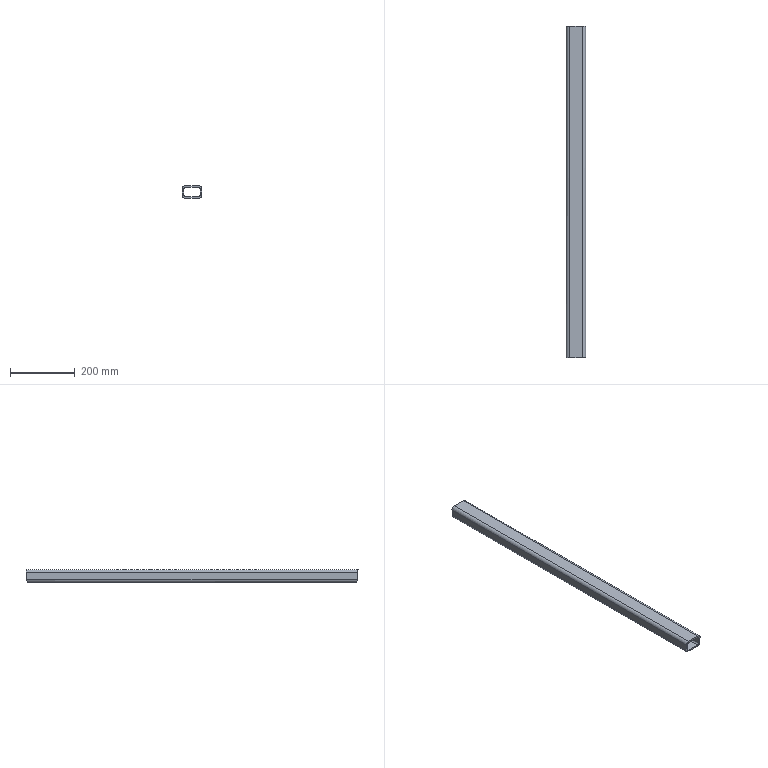Part | STEP file | body floor crossmember 1--000.001--20240926 | 1 solid | 18 faces | box 60 x 1025 x 40 mm | volume 853212 mm3 | plane 10 | cylinder 8 | commonest cylinder face diameters 10 x4 20 x4